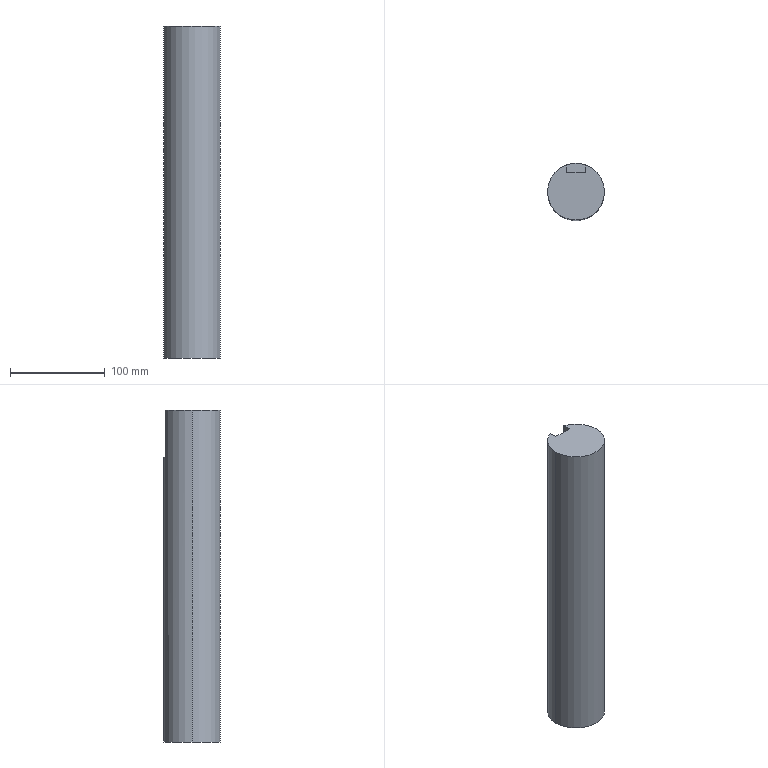Part | STEP file | 1 solid | 8 faces | box 60 x 60 x 350 mm | volume 980167 mm3 | plane 6 | cylinder 2 | commonest cylinder face diameters 60 x2
STEP:
#1=CARTESIAN_POINT('',(10.,28.284,183.));
#2=VERTEX_POINT('',#1);
#3=CARTESIAN_POINT('',(30.,0.,183.));
#4=VERTEX_POINT('',#3);
#5=CARTESIAN_POINT('',(0.,0.,183.));
#6=DIRECTION('',(0.,0.,-1.));
#7=DIRECTION('',(-1.,0.,0.));
#8=AXIS2_PLACEMENT_3D('',#5,#6,#7);
#9=CIRCLE('',#8,30.);
#10=EDGE_CURVE('',#2,#4,#9,.T.);
#11=ORIENTED_EDGE('',*,*,#10,.T.);
#12=CARTESIAN_POINT('',(30.,0.,-167.));
#13=VERTEX_POINT('',#12);
#14=CARTESIAN_POINT('',(30.,0.,183.));
#15=DIRECTION('',(0.,0.,-1.));
#16=VECTOR('',#15,1000.);
#17=LINE('',#14,#16);
#18=EDGE_CURVE('',#4,#13,#17,.T.);
#19=ORIENTED_EDGE('',*,*,#18,.T.);
#20=CARTESIAN_POINT('',(-30.,0.,-167.));
#21=VERTEX_POINT('',#20);
#22=CARTESIAN_POINT('',(0.,0.,-167.));
#23=DIRECTION('',(0.,0.,-1.));
#24=DIRECTION('',(-1.,0.,0.));
#25=AXIS2_PLACEMENT_3D('',#22,#23,#24);
#26=CIRCLE('',#25,30.);
#27=EDGE_CURVE('',#21,#13,#26,.T.);
#28=ORIENTED_EDGE('',*,*,#27,.F.);
#29=CARTESIAN_POINT('',(-30.,0.,183.));
#30=VERTEX_POINT('',#29);
#31=CARTESIAN_POINT('',(-30.,0.,183.));
#32=DIRECTION('',(0.,0.,-1.));
#33=VECTOR('',#32,1000.);
#34=LINE('',#31,#33);
#35=EDGE_CURVE('',#30,#21,#34,.T.);
#36=ORIENTED_EDGE('',*,*,#35,.F.);
#37=CARTESIAN_POINT('',(-10.,28.284,183.));
#38=VERTEX_POINT('',#37);
#39=CARTESIAN_POINT('',(0.,0.,183.));
#40=DIRECTION('',(0.,0.,-1.));
#41=DIRECTION('',(-1.,0.,0.));
#42=AXIS2_PLACEMENT_3D('',#39,#40,#41);
#43=CIRCLE('',#42,30.);
#44=EDGE_CURVE('',#30,#38,#43,.T.);
#45=ORIENTED_EDGE('',*,*,#44,.T.);
#46=CARTESIAN_POINT('',(-10.,28.284,133.));
#47=VERTEX_POINT('',#46);
#48=CARTESIAN_POINT('',(-10.,28.284,183.));
#49=DIRECTION('',(0.,0.,1.));
#50=VECTOR('',#49,1000.);
#51=LINE('',#48,#50);
#52=EDGE_CURVE('',#47,#38,#51,.T.);
#53=ORIENTED_EDGE('',*,*,#52,.F.);
#54=CARTESIAN_POINT('',(10.,28.284,133.));
#55=VERTEX_POINT('',#54);
#56=CARTESIAN_POINT('',(0.,0.,133.));
#57=DIRECTION('',(0.,0.,-1.));
#58=DIRECTION('',(1.,0.,0.));
#59=AXIS2_PLACEMENT_3D('',#56,#57,#58);
#60=CIRCLE('',#59,30.);
#61=EDGE_CURVE('',#47,#55,#60,.T.);
#62=ORIENTED_EDGE('',*,*,#61,.T.);
#63=CARTESIAN_POINT('',(10.,28.284,183.));
#64=DIRECTION('',(0.,0.,-1.));
#65=VECTOR('',#64,1000.);
#66=LINE('',#63,#65);
#67=EDGE_CURVE('',#2,#55,#66,.T.);
#68=ORIENTED_EDGE('',*,*,#67,.F.);
#69=EDGE_LOOP('',(#11,#19,#28,#36,#45,#53,#62,#68));
#70=FACE_OUTER_BOUND('',#69,.T.);
#71=CARTESIAN_POINT('',(0.,0.,183.));
#72=DIRECTION('',(0.,0.,-1.));
#73=DIRECTION('',(-1.,0.,0.));
#74=AXIS2_PLACEMENT_3D('',#71,#72,#73);
#75=CYLINDRICAL_SURFACE('',#74,30.);
#76=ADVANCED_FACE('',(#70),#75,.T.);
#77=ORIENTED_EDGE('',*,*,#18,.F.);
#78=CARTESIAN_POINT('',(0.,0.,183.));
#79=DIRECTION('',(0.,0.,-1.));
#80=DIRECTION('',(-1.,0.,0.));
#81=AXIS2_PLACEMENT_3D('',#78,#79,#80);
#82=CIRCLE('',#81,30.);
#83=EDGE_CURVE('',#4,#30,#82,.T.);
#84=ORIENTED_EDGE('',*,*,#83,.T.);
#85=ORIENTED_EDGE('',*,*,#35,.T.);
#86=CARTESIAN_POINT('',(0.,0.,-167.));
#87=DIRECTION('',(0.,0.,-1.));
#88=DIRECTION('',(-1.,0.,0.));
#89=AXIS2_PLACEMENT_3D('',#86,#87,#88);
#90=CIRCLE('',#89,30.);
#91=EDGE_CURVE('',#13,#21,#90,.T.);
#92=ORIENTED_EDGE('',*,*,#91,.F.);
#93=EDGE_LOOP('',(#77,#84,#85,#92));
#94=FACE_OUTER_BOUND('',#93,.T.);
#95=CARTESIAN_POINT('',(0.,0.,183.));
#96=DIRECTION('',(0.,0.,-1.));
#97=DIRECTION('',(-1.,0.,0.));
#98=AXIS2_PLACEMENT_3D('',#95,#96,#97);
#99=CYLINDRICAL_SURFACE('',#98,30.);
#100=ADVANCED_FACE('',(#94),#99,.T.);
#101=ORIENTED_EDGE('',*,*,#10,.F.);
#102=CARTESIAN_POINT('',(10.,20.,183.));
#103=VERTEX_POINT('',#102);
#104=CARTESIAN_POINT('',(10.,40.,183.));
#105=DIRECTION('',(0.,1.,0.));
#106=VECTOR('',#105,1000.);
#107=LINE('',#104,#106);
#108=EDGE_CURVE('',#103,#2,#107,.T.);
#109=ORIENTED_EDGE('',*,*,#108,.F.);
#110=CARTESIAN_POINT('',(-10.,20.,183.));
#111=VERTEX_POINT('',#110);
#112=CARTESIAN_POINT('',(-10.,20.,183.));
#113=DIRECTION('',(1.,0.,0.));
#114=VECTOR('',#113,1000.);
#115=LINE('',#112,#114);
#116=EDGE_CURVE('',#111,#103,#115,.T.);
#117=ORIENTED_EDGE('',*,*,#116,.F.);
#118=CARTESIAN_POINT('',(-10.,0.,183.));
#119=DIRECTION('',(0.,1.,0.));
#120=VECTOR('',#119,1000.);
#121=LINE('',#118,#120);
#122=EDGE_CURVE('',#111,#38,#121,.T.);
#123=ORIENTED_EDGE('',*,*,#122,.T.);
#124=ORIENTED_EDGE('',*,*,#44,.F.);
#125=ORIENTED_EDGE('',*,*,#83,.F.);
#126=EDGE_LOOP('',(#101,#109,#117,#123,#124,#125));
#127=FACE_OUTER_BOUND('',#126,.T.);
#128=CARTESIAN_POINT('',(0.,0.,183.));
#129=DIRECTION('',(0.,0.,-1.));
#130=DIRECTION('',(-1.,0.,0.));
#131=AXIS2_PLACEMENT_3D('',#128,#129,#130);
#132=PLANE('',#131);
#133=ADVANCED_FACE('',(#127),#132,.F.);
#134=ORIENTED_EDGE('',*,*,#27,.T.);
#135=ORIENTED_EDGE('',*,*,#91,.T.);
#136=EDGE_LOOP('',(#134,#135));
#137=FACE_OUTER_BOUND('',#136,.T.);
#138=CARTESIAN_POINT('',(0.,0.,-167.));
#139=DIRECTION('',(0.,0.,-1.));
#140=DIRECTION('',(-1.,0.,0.));
#141=AXIS2_PLACEMENT_3D('',#138,#139,#140);
#142=PLANE('',#141);
#143=ADVANCED_FACE('',(#137),#142,.T.);
#144=ORIENTED_EDGE('',*,*,#67,.T.);
#145=CARTESIAN_POINT('',(10.,20.,133.));
#146=VERTEX_POINT('',#145);
#147=CARTESIAN_POINT('',(10.,40.,133.));
#148=DIRECTION('',(0.,1.,0.));
#149=VECTOR('',#148,1000.);
#150=LINE('',#147,#149);
#151=EDGE_CURVE('',#146,#55,#150,.T.);
#152=ORIENTED_EDGE('',*,*,#151,.F.);
#153=CARTESIAN_POINT('',(10.,20.,133.));
#154=DIRECTION('',(0.,0.,1.));
#155=VECTOR('',#154,1000.);
#156=LINE('',#153,#155);
#157=EDGE_CURVE('',#146,#103,#156,.T.);
#158=ORIENTED_EDGE('',*,*,#157,.T.);
#159=ORIENTED_EDGE('',*,*,#108,.T.);
#160=EDGE_LOOP('',(#144,#152,#158,#159));
#161=FACE_OUTER_BOUND('',#160,.T.);
#162=CARTESIAN_POINT('',(10.,40.,133.));
#163=DIRECTION('',(1.,0.,0.));
#164=DIRECTION('',(0.,1.,0.));
#165=AXIS2_PLACEMENT_3D('',#162,#163,#164);
#166=PLANE('',#165);
#167=ADVANCED_FACE('',(#161),#166,.F.);
#168=ORIENTED_EDGE('',*,*,#116,.T.);
#169=ORIENTED_EDGE('',*,*,#157,.F.);
#170=CARTESIAN_POINT('',(-10.,20.,133.));
#171=VERTEX_POINT('',#170);
#172=CARTESIAN_POINT('',(-10.,20.,133.));
#173=DIRECTION('',(1.,0.,0.));
#174=VECTOR('',#173,1000.);
#175=LINE('',#172,#174);
#176=EDGE_CURVE('',#171,#146,#175,.T.);
#177=ORIENTED_EDGE('',*,*,#176,.F.);
#178=CARTESIAN_POINT('',(-10.,20.,133.));
#179=DIRECTION('',(0.,0.,1.));
#180=VECTOR('',#179,1000.);
#181=LINE('',#178,#180);
#182=EDGE_CURVE('',#171,#111,#181,.T.);
#183=ORIENTED_EDGE('',*,*,#182,.T.);
#184=EDGE_LOOP('',(#168,#169,#177,#183));
#185=FACE_OUTER_BOUND('',#184,.T.);
#186=CARTESIAN_POINT('',(-10.,20.,133.));
#187=DIRECTION('',(0.,-1.,0.));
#188=DIRECTION('',(0.,0.,-1.));
#189=AXIS2_PLACEMENT_3D('',#186,#187,#188);
#190=PLANE('',#189);
#191=ADVANCED_FACE('',(#185),#190,.F.);
#192=ORIENTED_EDGE('',*,*,#52,.T.);
#193=ORIENTED_EDGE('',*,*,#122,.F.);
#194=ORIENTED_EDGE('',*,*,#182,.F.);
#195=CARTESIAN_POINT('',(-10.,40.,133.));
#196=DIRECTION('',(0.,-1.,0.));
#197=VECTOR('',#196,1000.);
#198=LINE('',#195,#197);
#199=EDGE_CURVE('',#47,#171,#198,.T.);
#200=ORIENTED_EDGE('',*,*,#199,.F.);
#201=EDGE_LOOP('',(#192,#193,#194,#200));
#202=FACE_OUTER_BOUND('',#201,.T.);
#203=CARTESIAN_POINT('',(-10.,40.,133.));
#204=DIRECTION('',(-1.,0.,0.));
#205=DIRECTION('',(0.,-1.,0.));
#206=AXIS2_PLACEMENT_3D('',#203,#204,#205);
#207=PLANE('',#206);
#208=ADVANCED_FACE('',(#202),#207,.F.);
#209=ORIENTED_EDGE('',*,*,#199,.T.);
#210=ORIENTED_EDGE('',*,*,#176,.T.);
#211=ORIENTED_EDGE('',*,*,#151,.T.);
#212=ORIENTED_EDGE('',*,*,#61,.F.);
#213=EDGE_LOOP('',(#209,#210,#211,#212));
#214=FACE_OUTER_BOUND('',#213,.T.);
#215=CARTESIAN_POINT('',(0.,0.,133.));
#216=DIRECTION('',(0.,0.,1.));
#217=DIRECTION('',(1.,0.,0.));
#218=AXIS2_PLACEMENT_3D('',#215,#216,#217);
#219=PLANE('',#218);
#220=ADVANCED_FACE('',(#214),#219,.T.);
#221=CLOSED_SHELL('',(#76,#100,#133,#143,#167,#191,#208,#220));
#222=MANIFOLD_SOLID_BREP('',#221);
#223=CARTESIAN_POINT('',(0.,0.,0.));
#224=DIRECTION('',(0.,0.,1.));
#225=DIRECTION('',(1.,0.,0.));
#226=AXIS2_PLACEMENT_3D('',#223,#224,#225);
#227=(LENGTH_UNIT()NAMED_UNIT(*)SI_UNIT(.MILLI.,.METRE.));
#228=UNCERTAINTY_MEASURE_WITH_UNIT(LENGTH_MEASURE(0.00001),#227,'','');
#229=(NAMED_UNIT(*)PLANE_ANGLE_UNIT()SI_UNIT($,.RADIAN.));
#230=(NAMED_UNIT(*)SI_UNIT($,.STERADIAN.)SOLID_ANGLE_UNIT());
#231=(GEOMETRIC_REPRESENTATION_CONTEXT(3)GLOBAL_UNCERTAINTY_ASSIGNED_CONTEXT((#228))GLOBAL_UNIT_ASSIGNED_CONTEXT((#227,#229,#230))REPRESENTATION_CONTEXT('',''));
#232=ADVANCED_BREP_SHAPE_REPRESENTATION('',(#222,#226),#231);